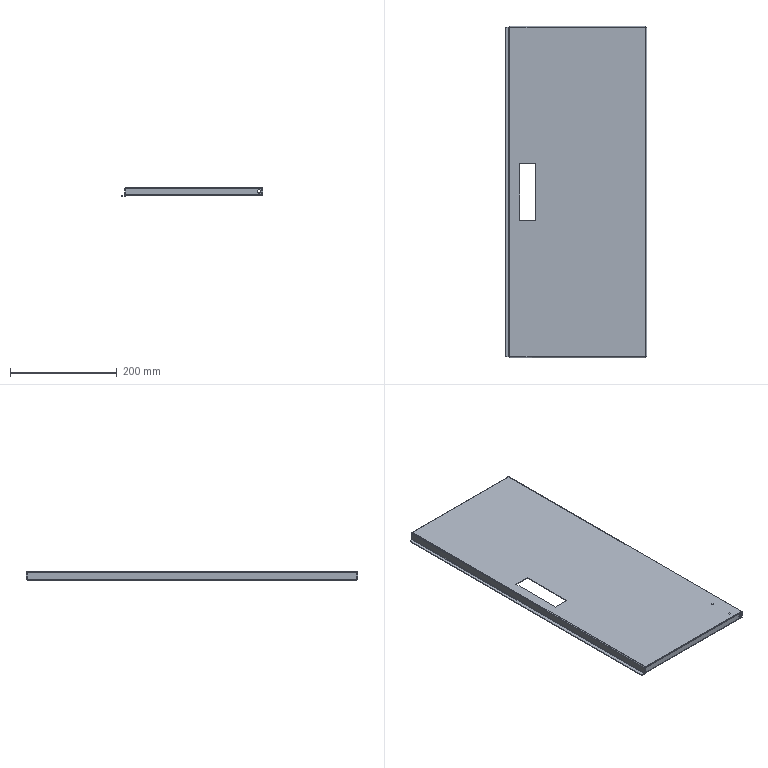Part | SolidWorks | features EdgeFlange 4, Fillet 2, ICE 2, SMBaseFlange 2, Cut 1, FlatPattern 1, LPattern 1, SheetMetal 1 | 1 solid | 92 faces | box 264.8 x 620 x 16 mm | volume 228976 mm3 | plane 56 | cylinder 28 | spline 8 | commonest cylinder face diameters 1.2 x5 3.6 x5 5 x4 6 x4 6.3 x4 1 x3